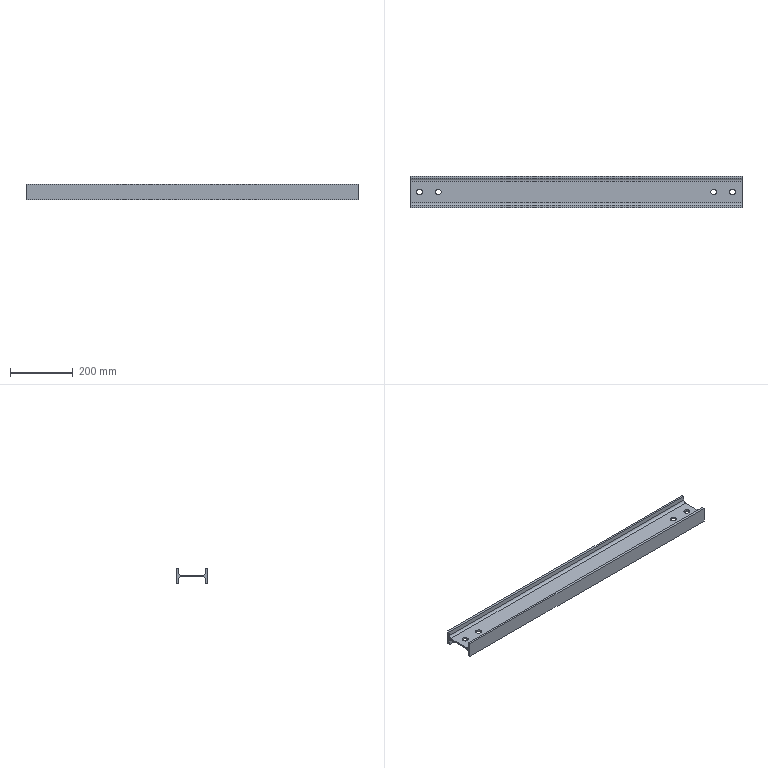Part | STEP file | 电柜辅梁3主体_Default<As Machined> | 1 solid | 26 faces | box 1058 x 100 x 50 mm | volume 1247401 mm3 | plane 14 | cylinder 12 | commonest cylinder face diameters 19 x8 16 x4